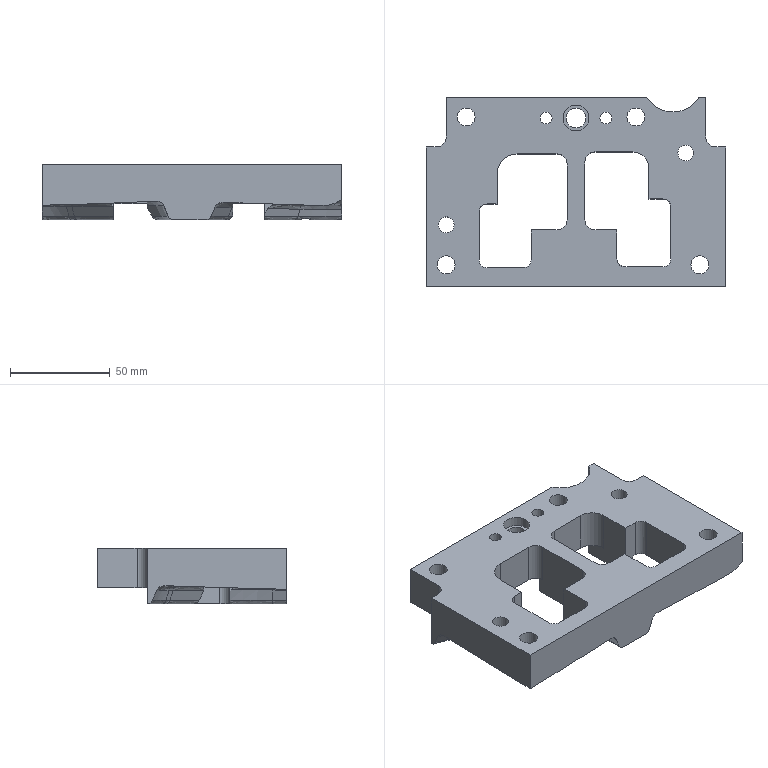Part | STEP file | 417_id1214_x_t | 1 solid | 119 faces | box 150 x 95 x 28 mm | volume 197794 mm3 | spline 44 | plane 44 | cylinder 31 | commonest cylinder face diameters 10 x9 8 x8 9 x4 14 x4 6 x2 13 x1